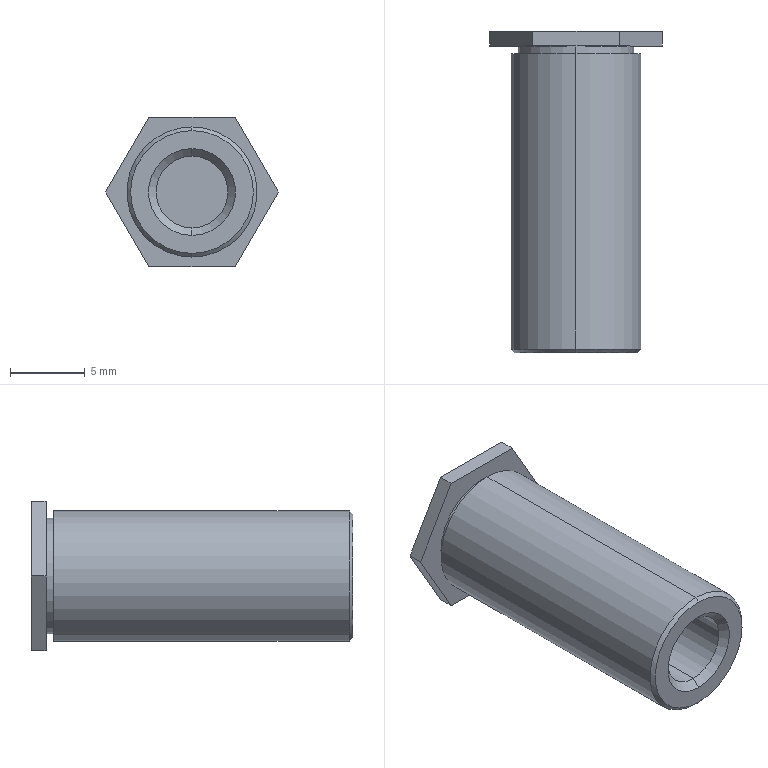Part | NX | features BREP 1 | 1 solid | 21 faces | box 11.547 x 21.5 x 10 mm | volume 934.056 mm3 | plane 11 | cylinder 6 | cone 4 | commonest cylinder face diameters 4.8 x2 7.7 x2 8.7 x2
STEP:
#1=CARTESIAN_POINT('',(0.,0.,-4.35));
#2=VERTEX_POINT('',#1);
#3=CARTESIAN_POINT('',(0.,0.,4.35));
#4=VERTEX_POINT('',#3);
#5=CARTESIAN_POINT('',(0.,0.,0.));
#6=DIRECTION('',(0.,-1.,0.));
#7=DIRECTION('',(0.,0.,-1.));
#8=AXIS2_PLACEMENT_3D('',#5,#6,#7);
#9=CIRCLE('',#8,4.35);
#10=EDGE_CURVE('',#2,#4,#9,.T.);
#11=ORIENTED_EDGE('',*,*,#10,.T.);
#12=CARTESIAN_POINT('',(0.,-19.75,4.35));
#13=VERTEX_POINT('',#12);
#14=CARTESIAN_POINT('',(0.,-13.,4.35));
#15=DIRECTION('',(0.,-1.,0.));
#16=VECTOR('',#15,1000.);
#17=LINE('',#14,#16);
#18=EDGE_CURVE('',#13,#4,#17,.F.);
#19=ORIENTED_EDGE('',*,*,#18,.F.);
#20=CARTESIAN_POINT('',(0.,-19.75,-4.35));
#21=VERTEX_POINT('',#20);
#22=CARTESIAN_POINT('',(0.,-19.75,0.));
#23=DIRECTION('',(0.,1.,0.));
#24=DIRECTION('',(0.,0.,-1.));
#25=AXIS2_PLACEMENT_3D('',#22,#23,#24);
#26=CIRCLE('',#25,4.35);
#27=EDGE_CURVE('',#13,#21,#26,.T.);
#28=ORIENTED_EDGE('',*,*,#27,.T.);
#29=CARTESIAN_POINT('',(0.,-13.,-4.35));
#30=DIRECTION('',(0.,-1.,0.));
#31=VECTOR('',#30,1000.);
#32=LINE('',#29,#31);
#33=EDGE_CURVE('',#21,#2,#32,.F.);
#34=ORIENTED_EDGE('',*,*,#33,.T.);
#35=EDGE_LOOP('',(#11,#19,#28,#34));
#36=FACE_BOUND('',#35,.T.);
#37=CARTESIAN_POINT('',(0.,-13.,0.));
#38=DIRECTION('',(0.,-1.,0.));
#39=DIRECTION('',(0.,0.,1.));
#40=AXIS2_PLACEMENT_3D('',#37,#38,#39);
#41=CYLINDRICAL_SURFACE('',#40,4.35);
#42=ADVANCED_FACE('',(#36),#41,.T.);
#43=CARTESIAN_POINT('',(0.,-20.,4.1));
#44=VERTEX_POINT('',#43);
#45=CARTESIAN_POINT('',(0.,-20.,-4.1));
#46=VERTEX_POINT('',#45);
#47=CARTESIAN_POINT('',(0.,-20.,0.));
#48=DIRECTION('',(0.,1.,0.));
#49=DIRECTION('',(0.,0.,1.));
#50=AXIS2_PLACEMENT_3D('',#47,#48,#49);
#51=CIRCLE('',#50,4.1);
#52=EDGE_CURVE('',#44,#46,#51,.T.);
#53=ORIENTED_EDGE('',*,*,#52,.T.);
#54=CARTESIAN_POINT('',(0.,-19.75,-4.35));
#55=DIRECTION('',(0.,0.7071,-0.7071));
#56=VECTOR('',#55,1000.);
#57=LINE('',#54,#56);
#58=EDGE_CURVE('',#46,#21,#57,.T.);
#59=ORIENTED_EDGE('',*,*,#58,.T.);
#60=ORIENTED_EDGE('',*,*,#27,.F.);
#61=CARTESIAN_POINT('',(0.,-19.75,4.35));
#62=DIRECTION('',(0.,0.7071,0.7071));
#63=VECTOR('',#62,1000.);
#64=LINE('',#61,#63);
#65=EDGE_CURVE('',#44,#13,#64,.T.);
#66=ORIENTED_EDGE('',*,*,#65,.F.);
#67=EDGE_LOOP('',(#53,#59,#60,#66));
#68=FACE_BOUND('',#67,.T.);
#69=CARTESIAN_POINT('',(0.,-19.75,0.));
#70=DIRECTION('',(0.,1.,0.));
#71=DIRECTION('',(0.,0.,-1.));
#72=AXIS2_PLACEMENT_3D('',#69,#70,#71);
#73=CONICAL_SURFACE('',#72,4.35,0.7854);
#74=ADVANCED_FACE('',(#68),#73,.T.);
#75=CARTESIAN_POINT('',(0.,0.5,-3.85));
#76=VERTEX_POINT('',#75);
#77=CARTESIAN_POINT('',(0.,0.5,3.85));
#78=VERTEX_POINT('',#77);
#79=CARTESIAN_POINT('',(0.,0.5,0.));
#80=DIRECTION('',(0.,-1.,0.));
#81=DIRECTION('',(0.,0.,-1.));
#82=AXIS2_PLACEMENT_3D('',#79,#80,#81);
#83=CIRCLE('',#82,3.85);
#84=EDGE_CURVE('',#76,#78,#83,.T.);
#85=ORIENTED_EDGE('',*,*,#84,.T.);
#86=CARTESIAN_POINT('',(0.,0.,3.85));
#87=VERTEX_POINT('',#86);
#88=CARTESIAN_POINT('',(0.,0.525,3.85));
#89=DIRECTION('',(0.,-1.,0.));
#90=VECTOR('',#89,1000.);
#91=LINE('',#88,#90);
#92=EDGE_CURVE('',#87,#78,#91,.F.);
#93=ORIENTED_EDGE('',*,*,#92,.F.);
#94=CARTESIAN_POINT('',(0.,0.,-3.85));
#95=VERTEX_POINT('',#94);
#96=CARTESIAN_POINT('',(0.,0.,0.));
#97=DIRECTION('',(0.,1.,0.));
#98=DIRECTION('',(0.,0.,-1.));
#99=AXIS2_PLACEMENT_3D('',#96,#97,#98);
#100=CIRCLE('',#99,3.85);
#101=EDGE_CURVE('',#87,#95,#100,.T.);
#102=ORIENTED_EDGE('',*,*,#101,.T.);
#103=CARTESIAN_POINT('',(0.,0.525,-3.85));
#104=DIRECTION('',(0.,-1.,0.));
#105=VECTOR('',#104,1000.);
#106=LINE('',#103,#105);
#107=EDGE_CURVE('',#95,#76,#106,.F.);
#108=ORIENTED_EDGE('',*,*,#107,.T.);
#109=EDGE_LOOP('',(#85,#93,#102,#108));
#110=FACE_BOUND('',#109,.T.);
#111=CARTESIAN_POINT('',(0.,0.525,0.));
#112=DIRECTION('',(0.,-1.,0.));
#113=DIRECTION('',(0.,0.,1.));
#114=AXIS2_PLACEMENT_3D('',#111,#112,#113);
#115=CYLINDRICAL_SURFACE('',#114,3.85);
#116=ADVANCED_FACE('',(#110),#115,.T.);
#117=CARTESIAN_POINT('',(0.,-19.5,2.4));
#118=VERTEX_POINT('',#117);
#119=CARTESIAN_POINT('',(0.,-19.5,-2.4));
#120=VERTEX_POINT('',#119);
#121=CARTESIAN_POINT('',(0.,-19.5,0.));
#122=DIRECTION('',(0.,-1.,0.));
#123=DIRECTION('',(0.,0.,-1.));
#124=AXIS2_PLACEMENT_3D('',#121,#122,#123);
#125=CIRCLE('',#124,2.4);
#126=EDGE_CURVE('',#118,#120,#125,.T.);
#127=ORIENTED_EDGE('',*,*,#126,.F.);
#128=CARTESIAN_POINT('',(0.,-20.,2.9));
#129=VERTEX_POINT('',#128);
#130=CARTESIAN_POINT('',(0.,-20.,2.9));
#131=DIRECTION('',(0.,-0.7071,0.7071));
#132=VECTOR('',#131,1000.);
#133=LINE('',#130,#132);
#134=EDGE_CURVE('',#129,#118,#133,.F.);
#135=ORIENTED_EDGE('',*,*,#134,.F.);
#136=CARTESIAN_POINT('',(0.,-20.,-2.9));
#137=VERTEX_POINT('',#136);
#138=CARTESIAN_POINT('',(0.,-20.,0.));
#139=DIRECTION('',(0.,-1.,0.));
#140=DIRECTION('',(0.,0.,-1.));
#141=AXIS2_PLACEMENT_3D('',#138,#139,#140);
#142=CIRCLE('',#141,2.9);
#143=EDGE_CURVE('',#129,#137,#142,.T.);
#144=ORIENTED_EDGE('',*,*,#143,.T.);
#145=CARTESIAN_POINT('',(0.,-20.,-2.9));
#146=DIRECTION('',(0.,-0.7071,-0.7071));
#147=VECTOR('',#146,1000.);
#148=LINE('',#145,#147);
#149=EDGE_CURVE('',#137,#120,#148,.F.);
#150=ORIENTED_EDGE('',*,*,#149,.T.);
#151=EDGE_LOOP('',(#127,#135,#144,#150));
#152=FACE_BOUND('',#151,.T.);
#153=CARTESIAN_POINT('',(0.,-20.,0.));
#154=DIRECTION('',(0.,-1.,0.));
#155=DIRECTION('',(0.,0.,1.));
#156=AXIS2_PLACEMENT_3D('',#153,#154,#155);
#157=CONICAL_SURFACE('',#156,2.9,0.7854);
#158=ADVANCED_FACE('',(#152),#157,.F.);
#159=ORIENTED_EDGE('',*,*,#126,.T.);
#160=CARTESIAN_POINT('',(0.,0.,-2.4));
#161=VERTEX_POINT('',#160);
#162=CARTESIAN_POINT('',(0.,0.,-2.4));
#163=DIRECTION('',(0.,1.,0.));
#164=VECTOR('',#163,1000.);
#165=LINE('',#162,#164);
#166=EDGE_CURVE('',#120,#161,#165,.T.);
#167=ORIENTED_EDGE('',*,*,#166,.T.);
#168=CARTESIAN_POINT('',(0.,0.,2.4));
#169=VERTEX_POINT('',#168);
#170=CARTESIAN_POINT('',(0.,0.,0.));
#171=DIRECTION('',(0.,-1.,0.));
#172=DIRECTION('',(0.,0.,1.));
#173=AXIS2_PLACEMENT_3D('',#170,#171,#172);
#174=CIRCLE('',#173,2.4);
#175=EDGE_CURVE('',#169,#161,#174,.T.);
#176=ORIENTED_EDGE('',*,*,#175,.F.);
#177=CARTESIAN_POINT('',(0.,0.,2.4));
#178=DIRECTION('',(0.,1.,0.));
#179=VECTOR('',#178,1000.);
#180=LINE('',#177,#179);
#181=EDGE_CURVE('',#118,#169,#180,.T.);
#182=ORIENTED_EDGE('',*,*,#181,.F.);
#183=EDGE_LOOP('',(#159,#167,#176,#182));
#184=FACE_BOUND('',#183,.T.);
#185=CARTESIAN_POINT('',(0.,0.,0.));
#186=DIRECTION('',(0.,1.,0.));
#187=DIRECTION('',(0.,0.,-1.));
#188=AXIS2_PLACEMENT_3D('',#185,#186,#187);
#189=CYLINDRICAL_SURFACE('',#188,2.4);
#190=ADVANCED_FACE('',(#184),#189,.F.);
#191=ORIENTED_EDGE('',*,*,#18,.T.);
#192=CARTESIAN_POINT('',(0.,0.,0.));
#193=DIRECTION('',(0.,-1.,0.));
#194=DIRECTION('',(0.,0.,-1.));
#195=AXIS2_PLACEMENT_3D('',#192,#193,#194);
#196=CIRCLE('',#195,4.35);
#197=EDGE_CURVE('',#4,#2,#196,.T.);
#198=ORIENTED_EDGE('',*,*,#197,.T.);
#199=ORIENTED_EDGE('',*,*,#33,.F.);
#200=CARTESIAN_POINT('',(0.,-19.75,0.));
#201=DIRECTION('',(0.,1.,0.));
#202=DIRECTION('',(0.,0.,-1.));
#203=AXIS2_PLACEMENT_3D('',#200,#201,#202);
#204=CIRCLE('',#203,4.35);
#205=EDGE_CURVE('',#21,#13,#204,.T.);
#206=ORIENTED_EDGE('',*,*,#205,.T.);
#207=EDGE_LOOP('',(#191,#198,#199,#206));
#208=FACE_BOUND('',#207,.T.);
#209=CARTESIAN_POINT('',(0.,-13.,0.));
#210=DIRECTION('',(0.,-1.,0.));
#211=DIRECTION('',(0.,0.,1.));
#212=AXIS2_PLACEMENT_3D('',#209,#210,#211);
#213=CYLINDRICAL_SURFACE('',#212,4.35);
#214=ADVANCED_FACE('',(#208),#213,.T.);
#215=ORIENTED_EDGE('',*,*,#58,.F.);
#216=CARTESIAN_POINT('',(0.,-20.,0.));
#217=DIRECTION('',(0.,1.,0.));
#218=DIRECTION('',(0.,0.,1.));
#219=AXIS2_PLACEMENT_3D('',#216,#217,#218);
#220=CIRCLE('',#219,4.1);
#221=EDGE_CURVE('',#46,#44,#220,.T.);
#222=ORIENTED_EDGE('',*,*,#221,.T.);
#223=ORIENTED_EDGE('',*,*,#65,.T.);
#224=ORIENTED_EDGE('',*,*,#205,.F.);
#225=EDGE_LOOP('',(#215,#222,#223,#224));
#226=FACE_BOUND('',#225,.T.);
#227=CARTESIAN_POINT('',(0.,-19.75,0.));
#228=DIRECTION('',(0.,1.,0.));
#229=DIRECTION('',(0.,0.,-1.));
#230=AXIS2_PLACEMENT_3D('',#227,#228,#229);
#231=CONICAL_SURFACE('',#230,4.35,0.7854);
#232=ADVANCED_FACE('',(#226),#231,.T.);
#233=ORIENTED_EDGE('',*,*,#10,.F.);
#234=ORIENTED_EDGE('',*,*,#197,.F.);
#235=EDGE_LOOP('',(#233,#234));
#236=FACE_BOUND('',#235,.T.);
#237=CARTESIAN_POINT('',(0.,0.,0.));
#238=DIRECTION('',(0.,1.,0.));
#239=DIRECTION('',(0.,0.,-1.));
#240=AXIS2_PLACEMENT_3D('',#237,#238,#239);
#241=CIRCLE('',#240,3.85);
#242=EDGE_CURVE('',#95,#87,#241,.T.);
#243=ORIENTED_EDGE('',*,*,#242,.F.);
#244=ORIENTED_EDGE('',*,*,#101,.F.);
#245=EDGE_LOOP('',(#243,#244));
#246=FACE_BOUND('',#245,.T.);
#247=CARTESIAN_POINT('',(0.,0.,0.));
#248=DIRECTION('',(0.,-1.,0.));
#249=DIRECTION('',(0.,0.,1.));
#250=AXIS2_PLACEMENT_3D('',#247,#248,#249);
#251=PLANE('',#250);
#252=ADVANCED_FACE('',(#236,#246),#251,.F.);
#253=ORIENTED_EDGE('',*,*,#52,.F.);
#254=ORIENTED_EDGE('',*,*,#221,.F.);
#255=EDGE_LOOP('',(#253,#254));
#256=FACE_BOUND('',#255,.T.);
#257=CARTESIAN_POINT('',(0.,-20.,0.));
#258=DIRECTION('',(0.,-1.,0.));
#259=DIRECTION('',(0.,0.,-1.));
#260=AXIS2_PLACEMENT_3D('',#257,#258,#259);
#261=CIRCLE('',#260,2.9);
#262=EDGE_CURVE('',#137,#129,#261,.T.);
#263=ORIENTED_EDGE('',*,*,#262,.F.);
#264=ORIENTED_EDGE('',*,*,#143,.F.);
#265=EDGE_LOOP('',(#263,#264));
#266=FACE_BOUND('',#265,.T.);
#267=CARTESIAN_POINT('',(1.375,-20.,-6.619));
#268=DIRECTION('',(0.,1.,0.));
#269=DIRECTION('',(0.,0.,-1.));
#270=AXIS2_PLACEMENT_3D('',#267,#268,#269);
#271=PLANE('',#270);
#272=ADVANCED_FACE('',(#256,#266),#271,.F.);
#273=ORIENTED_EDGE('',*,*,#92,.T.);
#274=CARTESIAN_POINT('',(0.,0.5,0.));
#275=DIRECTION('',(0.,-1.,0.));
#276=DIRECTION('',(0.,0.,-1.));
#277=AXIS2_PLACEMENT_3D('',#274,#275,#276);
#278=CIRCLE('',#277,3.85);
#279=EDGE_CURVE('',#78,#76,#278,.T.);
#280=ORIENTED_EDGE('',*,*,#279,.T.);
#281=ORIENTED_EDGE('',*,*,#107,.F.);
#282=ORIENTED_EDGE('',*,*,#242,.T.);
#283=EDGE_LOOP('',(#273,#280,#281,#282));
#284=FACE_BOUND('',#283,.T.);
#285=CARTESIAN_POINT('',(0.,0.525,0.));
#286=DIRECTION('',(0.,-1.,0.));
#287=DIRECTION('',(0.,0.,1.));
#288=AXIS2_PLACEMENT_3D('',#285,#286,#287);
#289=CYLINDRICAL_SURFACE('',#288,3.85);
#290=ADVANCED_FACE('',(#284),#289,.T.);
#291=ORIENTED_EDGE('',*,*,#134,.T.);
#292=CARTESIAN_POINT('',(0.,-19.5,0.));
#293=DIRECTION('',(0.,-1.,0.));
#294=DIRECTION('',(0.,0.,-1.));
#295=AXIS2_PLACEMENT_3D('',#292,#293,#294);
#296=CIRCLE('',#295,2.4);
#297=EDGE_CURVE('',#120,#118,#296,.T.);
#298=ORIENTED_EDGE('',*,*,#297,.F.);
#299=ORIENTED_EDGE('',*,*,#149,.F.);
#300=ORIENTED_EDGE('',*,*,#262,.T.);
#301=EDGE_LOOP('',(#291,#298,#299,#300));
#302=FACE_BOUND('',#301,.T.);
#303=CARTESIAN_POINT('',(0.,-20.,0.));
#304=DIRECTION('',(0.,-1.,0.));
#305=DIRECTION('',(0.,0.,1.));
#306=AXIS2_PLACEMENT_3D('',#303,#304,#305);
#307=CONICAL_SURFACE('',#306,2.9,0.7854);
#308=ADVANCED_FACE('',(#302),#307,.F.);
#309=CARTESIAN_POINT('',(2.887,0.5,-5.));
#310=VERTEX_POINT('',#309);
#311=CARTESIAN_POINT('',(-2.887,0.5,-5.));
#312=VERTEX_POINT('',#311);
#313=CARTESIAN_POINT('',(0.,0.5,-5.));
#314=DIRECTION('',(-1.,0.,0.));
#315=VECTOR('',#314,1000.);
#316=LINE('',#313,#315);
#317=EDGE_CURVE('',#310,#312,#316,.T.);
#318=ORIENTED_EDGE('',*,*,#317,.F.);
#319=CARTESIAN_POINT('',(5.774,0.5,0.));
#320=VERTEX_POINT('',#319);
#321=CARTESIAN_POINT('',(5.774,0.5,0.));
#322=DIRECTION('',(-0.5,0.,-0.866));
#323=VECTOR('',#322,1000.);
#324=LINE('',#321,#323);
#325=EDGE_CURVE('',#320,#310,#324,.T.);
#326=ORIENTED_EDGE('',*,*,#325,.F.);
#327=CARTESIAN_POINT('',(2.887,0.5,5.));
#328=VERTEX_POINT('',#327);
#329=CARTESIAN_POINT('',(2.887,0.5,5.));
#330=DIRECTION('',(0.5,0.,-0.866));
#331=VECTOR('',#330,1000.);
#332=LINE('',#329,#331);
#333=EDGE_CURVE('',#328,#320,#332,.T.);
#334=ORIENTED_EDGE('',*,*,#333,.F.);
#335=CARTESIAN_POINT('',(-2.887,0.5,5.));
#336=VERTEX_POINT('',#335);
#337=CARTESIAN_POINT('',(0.,0.5,5.));
#338=DIRECTION('',(1.,0.,0.));
#339=VECTOR('',#338,1000.);
#340=LINE('',#337,#339);
#341=EDGE_CURVE('',#336,#328,#340,.T.);
#342=ORIENTED_EDGE('',*,*,#341,.F.);
#343=CARTESIAN_POINT('',(-5.774,0.5,0.));
#344=VERTEX_POINT('',#343);
#345=CARTESIAN_POINT('',(-5.774,0.5,0.));
#346=DIRECTION('',(0.5,0.,0.866));
#347=VECTOR('',#346,1000.);
#348=LINE('',#345,#347);
#349=EDGE_CURVE('',#344,#336,#348,.T.);
#350=ORIENTED_EDGE('',*,*,#349,.F.);
#351=CARTESIAN_POINT('',(-2.887,0.5,-5.));
#352=DIRECTION('',(-0.5,0.,0.866));
#353=VECTOR('',#352,1000.);
#354=LINE('',#351,#353);
#355=EDGE_CURVE('',#312,#344,#354,.T.);
#356=ORIENTED_EDGE('',*,*,#355,.F.);
#357=EDGE_LOOP('',(#318,#326,#334,#342,#350,#356));
#358=FACE_BOUND('',#357,.T.);
#359=ORIENTED_EDGE('',*,*,#84,.F.);
#360=ORIENTED_EDGE('',*,*,#279,.F.);
#361=EDGE_LOOP('',(#359,#360));
#362=FACE_BOUND('',#361,.T.);
#363=CARTESIAN_POINT('',(0.,0.5,0.));
#364=DIRECTION('',(0.,1.,0.));
#365=DIRECTION('',(0.,0.,-1.));
#366=AXIS2_PLACEMENT_3D('',#363,#364,#365);
#367=PLANE('',#366);
#368=ADVANCED_FACE('',(#358,#362),#367,.F.);
#369=ORIENTED_EDGE('',*,*,#166,.F.);
#370=ORIENTED_EDGE('',*,*,#297,.T.);
#371=ORIENTED_EDGE('',*,*,#181,.T.);
#372=CARTESIAN_POINT('',(0.,0.,0.));
#373=DIRECTION('',(0.,-1.,0.));
#374=DIRECTION('',(0.,0.,1.));
#375=AXIS2_PLACEMENT_3D('',#372,#373,#374);
#376=CIRCLE('',#375,2.4);
#377=EDGE_CURVE('',#161,#169,#376,.T.);
#378=ORIENTED_EDGE('',*,*,#377,.F.);
#379=EDGE_LOOP('',(#369,#370,#371,#378));
#380=FACE_BOUND('',#379,.T.);
#381=CARTESIAN_POINT('',(0.,0.,0.));
#382=DIRECTION('',(0.,1.,0.));
#383=DIRECTION('',(0.,0.,-1.));
#384=AXIS2_PLACEMENT_3D('',#381,#382,#383);
#385=CYLINDRICAL_SURFACE('',#384,2.4);
#386=ADVANCED_FACE('',(#380),#385,.F.);
#387=CARTESIAN_POINT('',(-5.774,1.5,0.));
#388=VERTEX_POINT('',#387);
#389=CARTESIAN_POINT('',(-5.774,1.5,0.));
#390=DIRECTION('',(0.,1.,0.));
#391=VECTOR('',#390,1000.);
#392=LINE('',#389,#391);
#393=EDGE_CURVE('',#344,#388,#392,.T.);
#394=ORIENTED_EDGE('',*,*,#393,.T.);
#395=CARTESIAN_POINT('',(-2.887,1.5,-5.));
#396=VERTEX_POINT('',#395);
#397=CARTESIAN_POINT('',(-3.031,1.5,-4.75));
#398=DIRECTION('',(0.5,0.,-0.866));
#399=VECTOR('',#398,1000.);
#400=LINE('',#397,#399);
#401=EDGE_CURVE('',#388,#396,#400,.T.);
#402=ORIENTED_EDGE('',*,*,#401,.T.);
#403=CARTESIAN_POINT('',(-2.887,1.5,-5.));
#404=DIRECTION('',(0.,-1.,0.));
#405=VECTOR('',#404,1000.);
#406=LINE('',#403,#405);
#407=EDGE_CURVE('',#396,#312,#406,.T.);
#408=ORIENTED_EDGE('',*,*,#407,.T.);
#409=ORIENTED_EDGE('',*,*,#355,.T.);
#410=EDGE_LOOP('',(#394,#402,#408,#409));
#411=FACE_BOUND('',#410,.T.);
#412=CARTESIAN_POINT('',(-3.031,1.5,-4.75));
#413=DIRECTION('',(-0.866,0.,-0.5));
#414=DIRECTION('',(0.5,0.,-0.866));
#415=AXIS2_PLACEMENT_3D('',#412,#413,#414);
#416=PLANE('',#415);
#417=ADVANCED_FACE('',(#411),#416,.T.);
#418=ORIENTED_EDGE('',*,*,#407,.F.);
#419=CARTESIAN_POINT('',(2.887,1.5,-5.));
#420=VERTEX_POINT('',#419);
#421=CARTESIAN_POINT('',(2.598,1.5,-5.));
#422=DIRECTION('',(1.,0.,0.));
#423=VECTOR('',#422,1000.);
#424=LINE('',#421,#423);
#425=EDGE_CURVE('',#396,#420,#424,.T.);
#426=ORIENTED_EDGE('',*,*,#425,.T.);
#427=CARTESIAN_POINT('',(2.887,1.5,-5.));
#428=DIRECTION('',(0.,-1.,0.));
#429=VECTOR('',#428,1000.);
#430=LINE('',#427,#429);
#431=EDGE_CURVE('',#420,#310,#430,.T.);
#432=ORIENTED_EDGE('',*,*,#431,.T.);
#433=ORIENTED_EDGE('',*,*,#317,.T.);
#434=EDGE_LOOP('',(#418,#426,#432,#433));
#435=FACE_BOUND('',#434,.T.);
#436=CARTESIAN_POINT('',(2.598,1.5,-5.));
#437=DIRECTION('',(0.,0.,-1.));
#438=DIRECTION('',(1.,0.,0.));
#439=AXIS2_PLACEMENT_3D('',#436,#437,#438);
#440=PLANE('',#439);
#441=ADVANCED_FACE('',(#435),#440,.T.);
#442=ORIENTED_EDGE('',*,*,#431,.F.);
#443=CARTESIAN_POINT('',(5.774,1.5,0.));
#444=VERTEX_POINT('',#443);
#445=CARTESIAN_POINT('',(5.629,1.5,-0.25));
#446=DIRECTION('',(0.5,0.,0.866));
#447=VECTOR('',#446,1000.);
#448=LINE('',#445,#447);
#449=EDGE_CURVE('',#420,#444,#448,.T.);
#450=ORIENTED_EDGE('',*,*,#449,.T.);
#451=CARTESIAN_POINT('',(5.774,1.5,0.));
#452=DIRECTION('',(0.,-1.,0.));
#453=VECTOR('',#452,1000.);
#454=LINE('',#451,#453);
#455=EDGE_CURVE('',#444,#320,#454,.T.);
#456=ORIENTED_EDGE('',*,*,#455,.T.);
#457=ORIENTED_EDGE('',*,*,#325,.T.);
#458=EDGE_LOOP('',(#442,#450,#456,#457));
#459=FACE_BOUND('',#458,.T.);
#460=CARTESIAN_POINT('',(5.629,1.5,-0.25));
#461=DIRECTION('',(0.866,0.,-0.5));
#462=DIRECTION('',(0.5,0.,0.866));
#463=AXIS2_PLACEMENT_3D('',#460,#461,#462);
#464=PLANE('',#463);
#465=ADVANCED_FACE('',(#459),#464,.T.);
#466=ORIENTED_EDGE('',*,*,#455,.F.);
#467=CARTESIAN_POINT('',(2.887,1.5,5.));
#468=VERTEX_POINT('',#467);
#469=CARTESIAN_POINT('',(3.031,1.5,4.75));
#470=DIRECTION('',(-0.5,0.,0.866));
#471=VECTOR('',#470,1000.);
#472=LINE('',#469,#471);
#473=EDGE_CURVE('',#444,#468,#472,.T.);
#474=ORIENTED_EDGE('',*,*,#473,.T.);
#475=CARTESIAN_POINT('',(2.887,1.5,5.));
#476=DIRECTION('',(0.,-1.,0.));
#477=VECTOR('',#476,1000.);
#478=LINE('',#475,#477);
#479=EDGE_CURVE('',#468,#328,#478,.T.);
#480=ORIENTED_EDGE('',*,*,#479,.T.);
#481=ORIENTED_EDGE('',*,*,#333,.T.);
#482=EDGE_LOOP('',(#466,#474,#480,#481));
#483=FACE_BOUND('',#482,.T.);
#484=CARTESIAN_POINT('',(3.031,1.5,4.75));
#485=DIRECTION('',(0.866,0.,0.5));
#486=DIRECTION('',(-0.5,0.,0.866));
#487=AXIS2_PLACEMENT_3D('',#484,#485,#486);
#488=PLANE('',#487);
#489=ADVANCED_FACE('',(#483),#488,.T.);
#490=ORIENTED_EDGE('',*,*,#479,.F.);
#491=CARTESIAN_POINT('',(-2.887,1.5,5.));
#492=VERTEX_POINT('',#491);
#493=CARTESIAN_POINT('',(-2.598,1.5,5.));
#494=DIRECTION('',(-1.,0.,0.));
#495=VECTOR('',#494,1000.);
#496=LINE('',#493,#495);
#497=EDGE_CURVE('',#468,#492,#496,.T.);
#498=ORIENTED_EDGE('',*,*,#497,.T.);
#499=CARTESIAN_POINT('',(-2.887,1.5,5.));
#500=DIRECTION('',(0.,-1.,0.));
#501=VECTOR('',#500,1000.);
#502=LINE('',#499,#501);
#503=EDGE_CURVE('',#492,#336,#502,.T.);
#504=ORIENTED_EDGE('',*,*,#503,.T.);
#505=ORIENTED_EDGE('',*,*,#341,.T.);
#506=EDGE_LOOP('',(#490,#498,#504,#505));
#507=FACE_BOUND('',#506,.T.);
#508=CARTESIAN_POINT('',(-2.598,1.5,5.));
#509=DIRECTION('',(0.,0.,1.));
#510=DIRECTION('',(-1.,0.,0.));
#511=AXIS2_PLACEMENT_3D('',#508,#509,#510);
#512=PLANE('',#511);
#513=ADVANCED_FACE('',(#507),#512,.T.);
#514=ORIENTED_EDGE('',*,*,#503,.F.);
#515=CARTESIAN_POINT('',(-5.629,1.5,0.25));
#516=DIRECTION('',(-0.5,0.,-0.866));
#517=VECTOR('',#516,1000.);
#518=LINE('',#515,#517);
#519=EDGE_CURVE('',#492,#388,#518,.T.);
#520=ORIENTED_EDGE('',*,*,#519,.T.);
#521=ORIENTED_EDGE('',*,*,#393,.F.);
#522=ORIENTED_EDGE('',*,*,#349,.T.);
#523=EDGE_LOOP('',(#514,#520,#521,#522));
#524=FACE_BOUND('',#523,.T.);
#525=CARTESIAN_POINT('',(-5.629,1.5,0.25));
#526=DIRECTION('',(-0.866,0.,0.5));
#527=DIRECTION('',(-0.5,0.,-0.866));
#528=AXIS2_PLACEMENT_3D('',#525,#526,#527);
#529=PLANE('',#528);
#530=ADVANCED_FACE('',(#524),#529,.T.);
#531=ORIENTED_EDGE('',*,*,#175,.T.);
#532=ORIENTED_EDGE('',*,*,#377,.T.);
#533=EDGE_LOOP('',(#531,#532));
#534=FACE_BOUND('',#533,.T.);
#535=CARTESIAN_POINT('',(0.,0.,0.));
#536=DIRECTION('',(0.,-1.,0.));
#537=DIRECTION('',(0.,0.,1.));
#538=AXIS2_PLACEMENT_3D('',#535,#536,#537);
#539=PLANE('',#538);
#540=ADVANCED_FACE('',(#534),#539,.T.);
#541=ORIENTED_EDGE('',*,*,#425,.F.);
#542=ORIENTED_EDGE('',*,*,#401,.F.);
#543=ORIENTED_EDGE('',*,*,#519,.F.);
#544=ORIENTED_EDGE('',*,*,#497,.F.);
#545=ORIENTED_EDGE('',*,*,#473,.F.);
#546=ORIENTED_EDGE('',*,*,#449,.F.);
#547=EDGE_LOOP('',(#541,#542,#543,#544,#545,#546));
#548=FACE_BOUND('',#547,.T.);
#549=CARTESIAN_POINT('',(0.,1.5,0.));
#550=DIRECTION('',(0.,1.,0.));
#551=DIRECTION('',(0.,0.,-1.));
#552=AXIS2_PLACEMENT_3D('',#549,#550,#551);
#553=PLANE('',#552);
#554=ADVANCED_FACE('',(#548),#553,.T.);
#555=CLOSED_SHELL('',(#42,#74,#116,#158,#190,#214,#232,#252,#272,#290,#308,#368,#386,#417,#441,#465,#489,#513,#530,#540,#554));
#556=MANIFOLD_SOLID_BREP('',#555);
#557=(LENGTH_UNIT()NAMED_UNIT(*)SI_UNIT(.MILLI.,.METRE.));
#558=UNCERTAINTY_MEASURE_WITH_UNIT(LENGTH_MEASURE(0.00001),#557,'','');
#559=(NAMED_UNIT(*)PLANE_ANGLE_UNIT()SI_UNIT($,.RADIAN.));
#560=(NAMED_UNIT(*)SI_UNIT($,.STERADIAN.)SOLID_ANGLE_UNIT());
#561=(GEOMETRIC_REPRESENTATION_CONTEXT(3)GLOBAL_UNCERTAINTY_ASSIGNED_CONTEXT((#558))GLOBAL_UNIT_ASSIGNED_CONTEXT((#557,#559,#560))REPRESENTATION_CONTEXT('',''));
#562=ADVANCED_BREP_SHAPE_REPRESENTATION('',(#556),#561);